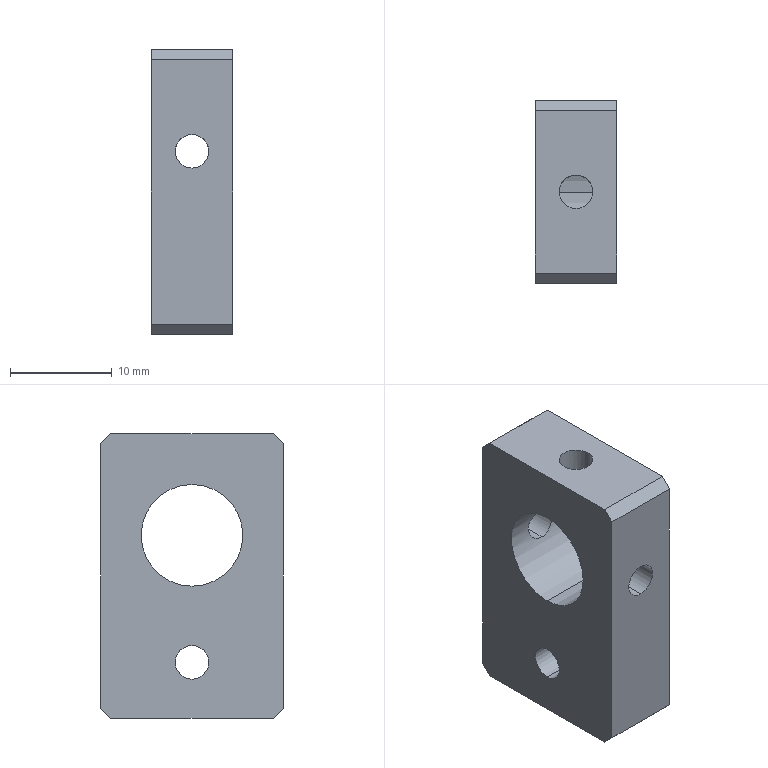Part | SolidWorks | features HoleWzd 3, Chamfer 1, Extrusion 1, ICE 1 | 1 solid | 20 faces | box 8 x 18 x 28 mm | volume 3206 mm3 | cylinder 10 | plane 10 | commonest cylinder face diameters 3.3 x8 10 x2
STEP:
#1=CARTESIAN_POINT('',(0.,-9.,2.35));
#2=VERTEX_POINT('',#1);
#3=CARTESIAN_POINT('',(0.,-9.,5.65));
#4=VERTEX_POINT('',#3);
#5=CARTESIAN_POINT('',(0.,-9.,4.));
#6=DIRECTION('',(0.,1.,0.));
#7=DIRECTION('',(0.,0.,1.));
#8=AXIS2_PLACEMENT_3D('',#5,#6,#7);
#9=CIRCLE('',#8,1.65);
#10=EDGE_CURVE('',#2,#4,#9,.T.);
#11=ORIENTED_EDGE('',*,*,#10,.F.);
#12=CARTESIAN_POINT('',(0.,-4.72,2.35));
#13=VERTEX_POINT('',#12);
#14=CARTESIAN_POINT('',(0.,9.,2.35));
#15=DIRECTION('',(0.,1.,0.));
#16=VECTOR('',#15,1000.);
#17=LINE('',#14,#16);
#18=EDGE_CURVE('',#2,#13,#17,.T.);
#19=ORIENTED_EDGE('',*,*,#18,.T.);
#20=CARTESIAN_POINT('',(0.,-4.72,5.65));
#21=VERTEX_POINT('',#20);
#22=CARTESIAN_POINT('',(0.,-4.72,5.65));
#23=CARTESIAN_POINT('',(-0.1099,-4.72,5.65));
#24=CARTESIAN_POINT('',(-0.2177,-4.724,5.639));
#25=CARTESIAN_POINT('',(-0.4296,-4.738,5.597));
#26=CARTESIAN_POINT('',(-0.5348,-4.749,5.565));
#27=CARTESIAN_POINT('',(-0.7342,-4.776,5.482));
#28=CARTESIAN_POINT('',(-0.8287,-4.791,5.431));
#29=CARTESIAN_POINT('',(-1.007,-4.825,5.311));
#30=CARTESIAN_POINT('',(-1.091,-4.844,5.242));
#31=CARTESIAN_POINT('',(-1.318,-4.898,5.015));
#32=CARTESIAN_POINT('',(-1.441,-4.934,4.833));
#33=CARTESIAN_POINT('',(-1.565,-4.972,4.535));
#34=CARTESIAN_POINT('',(-1.597,-4.983,4.43));
#35=CARTESIAN_POINT('',(-1.639,-4.996,4.217));
#36=CARTESIAN_POINT('',(-1.65,-5.,4.109));
#37=CARTESIAN_POINT('',(-1.65,-5.,3.892));
#38=CARTESIAN_POINT('',(-1.639,-4.996,3.782));
#39=CARTESIAN_POINT('',(-1.597,-4.983,3.57));
#40=CARTESIAN_POINT('',(-1.565,-4.972,3.466));
#41=CARTESIAN_POINT('',(-1.44,-4.934,3.165));
#42=CARTESIAN_POINT('',(-1.318,-4.898,2.984));
#43=CARTESIAN_POINT('',(-1.09,-4.844,2.757));
#44=CARTESIAN_POINT('',(-1.007,-4.825,2.689));
#45=CARTESIAN_POINT('',(-0.8292,-4.791,2.569));
#46=CARTESIAN_POINT('',(-0.7327,-4.775,2.518));
#47=CARTESIAN_POINT('',(-0.5341,-4.749,2.435));
#48=CARTESIAN_POINT('',(-0.4311,-4.738,2.404));
#49=CARTESIAN_POINT('',(-0.2176,-4.724,2.361));
#50=CARTESIAN_POINT('',(-0.1082,-4.72,2.35));
#51=CARTESIAN_POINT('',(0.,-4.72,2.35));
#52=B_SPLINE_CURVE_WITH_KNOTS('',3,(#22,#23,#24,#25,#26,#27,#28,#29,#30,#31,#32,#33,#34,#35,#36,#37,#38,#39,#40,#41,#42,#43,#44,#45,#46,#47,#48,#49,#50,#51),.UNSPECIFIED.,.F.,.F.,(4,2,2,2,2,2,2,2,2,2,2,2,2,2,4),(0.,0.0003247,0.0006494,0.0009741,0.001299,0.001948,0.002273,0.002598,0.002922,0.003247,0.003896,0.004221,0.004546,0.00487,0.005195),.UNSPECIFIED.);
#53=EDGE_CURVE('',#21,#13,#52,.T.);
#54=ORIENTED_EDGE('',*,*,#53,.F.);
#55=CARTESIAN_POINT('',(0.,9.,5.65));
#56=DIRECTION('',(0.,1.,0.));
#57=VECTOR('',#56,1000.);
#58=LINE('',#55,#57);
#59=EDGE_CURVE('',#4,#21,#58,.T.);
#60=ORIENTED_EDGE('',*,*,#59,.F.);
#61=EDGE_LOOP('',(#11,#19,#54,#60));
#62=FACE_OUTER_BOUND('',#61,.T.);
#63=CARTESIAN_POINT('',(0.,9.,4.));
#64=DIRECTION('',(0.,1.,0.));
#65=DIRECTION('',(0.,0.,1.));
#66=AXIS2_PLACEMENT_3D('',#63,#64,#65);
#67=CYLINDRICAL_SURFACE('',#66,1.65);
#68=ADVANCED_FACE('',(#62),#67,.F.);
#69=CARTESIAN_POINT('',(0.,4.72,2.35));
#70=VERTEX_POINT('',#69);
#71=CARTESIAN_POINT('',(0.,4.72,5.65));
#72=VERTEX_POINT('',#71);
#73=CARTESIAN_POINT('',(0.,4.72,2.35));
#74=CARTESIAN_POINT('',(-0.2163,4.72,2.35));
#75=CARTESIAN_POINT('',(-0.4347,4.736,2.394));
#76=CARTESIAN_POINT('',(-0.7332,4.776,2.518));
#77=CARTESIAN_POINT('',(-0.8297,4.791,2.57));
#78=CARTESIAN_POINT('',(-1.008,4.826,2.689));
#79=CARTESIAN_POINT('',(-1.09,4.844,2.757));
#80=CARTESIAN_POINT('',(-1.319,4.899,2.986));
#81=CARTESIAN_POINT('',(-1.44,4.934,3.166));
#82=CARTESIAN_POINT('',(-1.565,4.972,3.467));
#83=CARTESIAN_POINT('',(-1.597,4.983,3.57));
#84=CARTESIAN_POINT('',(-1.639,4.996,3.781));
#85=CARTESIAN_POINT('',(-1.65,5.,3.891));
#86=CARTESIAN_POINT('',(-1.65,5.,4.109));
#87=CARTESIAN_POINT('',(-1.639,4.996,4.217));
#88=CARTESIAN_POINT('',(-1.597,4.983,4.43));
#89=CARTESIAN_POINT('',(-1.565,4.972,4.535));
#90=CARTESIAN_POINT('',(-1.441,4.934,4.833));
#91=CARTESIAN_POINT('',(-1.318,4.898,5.016));
#92=CARTESIAN_POINT('',(-1.091,4.844,5.242));
#93=CARTESIAN_POINT('',(-1.007,4.825,5.312));
#94=CARTESIAN_POINT('',(-0.8285,4.791,5.431));
#95=CARTESIAN_POINT('',(-0.7342,4.776,5.482));
#96=CARTESIAN_POINT('',(-0.5349,4.749,5.565));
#97=CARTESIAN_POINT('',(-0.4296,4.738,5.597));
#98=CARTESIAN_POINT('',(-0.2177,4.724,5.639));
#99=CARTESIAN_POINT('',(-0.1098,4.72,5.65));
#100=CARTESIAN_POINT('',(0.,4.72,5.65));
#101=B_SPLINE_CURVE_WITH_KNOTS('',3,(#73,#74,#75,#76,#77,#78,#79,#80,#81,#82,#83,#84,#85,#86,#87,#88,#89,#90,#91,#92,#93,#94,#95,#96,#97,#98,#99,#100),.UNSPECIFIED.,.F.,.F.,(4,2,2,2,2,2,2,2,2,2,2,2,2,4),(0.005195,0.005844,0.006169,0.006494,0.007143,0.007467,0.007792,0.008117,0.008441,0.009091,0.009415,0.00974,0.01006,0.01039),.UNSPECIFIED.);
#102=EDGE_CURVE('',#70,#72,#101,.T.);
#103=ORIENTED_EDGE('',*,*,#102,.F.);
#104=CARTESIAN_POINT('',(0.,9.,2.35));
#105=VERTEX_POINT('',#104);
#106=CARTESIAN_POINT('',(0.,9.,2.35));
#107=DIRECTION('',(0.,1.,0.));
#108=VECTOR('',#107,1000.);
#109=LINE('',#106,#108);
#110=EDGE_CURVE('',#70,#105,#109,.T.);
#111=ORIENTED_EDGE('',*,*,#110,.T.);
#112=CARTESIAN_POINT('',(0.,9.,5.65));
#113=VERTEX_POINT('',#112);
#114=CARTESIAN_POINT('',(0.,9.,4.));
#115=DIRECTION('',(0.,1.,0.));
#116=DIRECTION('',(0.,0.,1.));
#117=AXIS2_PLACEMENT_3D('',#114,#115,#116);
#118=CIRCLE('',#117,1.65);
#119=EDGE_CURVE('',#105,#113,#118,.T.);
#120=ORIENTED_EDGE('',*,*,#119,.T.);
#121=CARTESIAN_POINT('',(0.,9.,5.65));
#122=DIRECTION('',(0.,1.,0.));
#123=VECTOR('',#122,1000.);
#124=LINE('',#121,#123);
#125=EDGE_CURVE('',#72,#113,#124,.T.);
#126=ORIENTED_EDGE('',*,*,#125,.F.);
#127=EDGE_LOOP('',(#103,#111,#120,#126));
#128=FACE_OUTER_BOUND('',#127,.T.);
#129=CARTESIAN_POINT('',(0.,9.,4.));
#130=DIRECTION('',(0.,1.,0.));
#131=DIRECTION('',(0.,0.,1.));
#132=AXIS2_PLACEMENT_3D('',#129,#130,#131);
#133=CYLINDRICAL_SURFACE('',#132,1.65);
#134=ADVANCED_FACE('',(#128),#133,.F.);
#135=CARTESIAN_POINT('',(-4.,0.,-6.85));
#136=VERTEX_POINT('',#135);
#137=CARTESIAN_POINT('',(-4.,0.,-10.15));
#138=VERTEX_POINT('',#137);
#139=CARTESIAN_POINT('',(-4.,0.,-8.5));
#140=DIRECTION('',(1.,0.,0.));
#141=DIRECTION('',(0.,0.,-1.));
#142=AXIS2_PLACEMENT_3D('',#139,#140,#141);
#143=CIRCLE('',#142,1.65);
#144=EDGE_CURVE('',#136,#138,#143,.T.);
#145=ORIENTED_EDGE('',*,*,#144,.F.);
#146=CARTESIAN_POINT('',(4.,0.,-6.85));
#147=VERTEX_POINT('',#146);
#148=CARTESIAN_POINT('',(4.,0.,-6.85));
#149=DIRECTION('',(1.,0.,0.));
#150=VECTOR('',#149,1000.);
#151=LINE('',#148,#150);
#152=EDGE_CURVE('',#136,#147,#151,.T.);
#153=ORIENTED_EDGE('',*,*,#152,.T.);
#154=CARTESIAN_POINT('',(4.,0.,-10.15));
#155=VERTEX_POINT('',#154);
#156=CARTESIAN_POINT('',(4.,0.,-8.5));
#157=DIRECTION('',(1.,0.,0.));
#158=DIRECTION('',(0.,0.,-1.));
#159=AXIS2_PLACEMENT_3D('',#156,#157,#158);
#160=CIRCLE('',#159,1.65);
#161=EDGE_CURVE('',#147,#155,#160,.T.);
#162=ORIENTED_EDGE('',*,*,#161,.T.);
#163=CARTESIAN_POINT('',(4.,0.,-10.15));
#164=DIRECTION('',(1.,0.,0.));
#165=VECTOR('',#164,1000.);
#166=LINE('',#163,#165);
#167=EDGE_CURVE('',#138,#155,#166,.T.);
#168=ORIENTED_EDGE('',*,*,#167,.F.);
#169=EDGE_LOOP('',(#145,#153,#162,#168));
#170=FACE_OUTER_BOUND('',#169,.T.);
#171=CARTESIAN_POINT('',(4.,0.,-8.5));
#172=DIRECTION('',(1.,0.,0.));
#173=DIRECTION('',(0.,0.,-1.));
#174=AXIS2_PLACEMENT_3D('',#171,#172,#173);
#175=CYLINDRICAL_SURFACE('',#174,1.65);
#176=ADVANCED_FACE('',(#170),#175,.F.);
#177=CARTESIAN_POINT('',(-1.65,0.,9.));
#178=VERTEX_POINT('',#177);
#179=CARTESIAN_POINT('',(1.65,0.,9.));
#180=VERTEX_POINT('',#179);
#181=CARTESIAN_POINT('',(-1.65,0.,9.));
#182=CARTESIAN_POINT('',(-1.65,-0.2164,9.));
#183=CARTESIAN_POINT('',(-1.606,-0.4348,8.985));
#184=CARTESIAN_POINT('',(-1.482,-0.7334,8.947));
#185=CARTESIAN_POINT('',(-1.43,-0.8299,8.931));
#186=CARTESIAN_POINT('',(-1.311,-1.008,8.898));
#187=CARTESIAN_POINT('',(-1.243,-1.091,8.88));
#188=CARTESIAN_POINT('',(-1.014,-1.319,8.825));
#189=CARTESIAN_POINT('',(-0.8342,-1.44,8.789));
#190=CARTESIAN_POINT('',(-0.5334,-1.565,8.749));
#191=CARTESIAN_POINT('',(-0.4303,-1.597,8.738));
#192=CARTESIAN_POINT('',(-0.2186,-1.639,8.724));
#193=CARTESIAN_POINT('',(-0.1086,-1.65,8.72));
#194=CARTESIAN_POINT('',(0.1089,-1.65,8.72));
#195=CARTESIAN_POINT('',(0.2165,-1.639,8.724));
#196=CARTESIAN_POINT('',(0.4297,-1.597,8.738));
#197=CARTESIAN_POINT('',(0.5347,-1.565,8.749));
#198=CARTESIAN_POINT('',(0.8327,-1.441,8.789));
#199=CARTESIAN_POINT('',(1.015,-1.318,8.826));
#200=CARTESIAN_POINT('',(1.242,-1.091,8.88));
#201=CARTESIAN_POINT('',(1.311,-1.007,8.898));
#202=CARTESIAN_POINT('',(1.431,-0.8287,8.932));
#203=CARTESIAN_POINT('',(1.481,-0.7344,8.947));
#204=CARTESIAN_POINT('',(1.565,-0.535,8.972));
#205=CARTESIAN_POINT('',(1.597,-0.4297,8.983));
#206=CARTESIAN_POINT('',(1.639,-0.2177,8.996));
#207=CARTESIAN_POINT('',(1.65,-0.1098,9.));
#208=CARTESIAN_POINT('',(1.65,0.,9.));
#209=B_SPLINE_CURVE_WITH_KNOTS('',3,(#181,#182,#183,#184,#185,#186,#187,#188,#189,#190,#191,#192,#193,#194,#195,#196,#197,#198,#199,#200,#201,#202,#203,#204,#205,#206,#207,#208),.UNSPECIFIED.,.F.,.F.,(4,2,2,2,2,2,2,2,2,2,2,2,2,4),(0.005195,0.005845,0.006169,0.006494,0.007143,0.007468,0.007792,0.008117,0.008442,0.009091,0.009415,0.00974,0.01006,0.01039),.UNSPECIFIED.);
#210=EDGE_CURVE('',#178,#180,#209,.T.);
#211=ORIENTED_EDGE('',*,*,#210,.F.);
#212=CARTESIAN_POINT('',(-1.65,0.,14.));
#213=VERTEX_POINT('',#212);
#214=CARTESIAN_POINT('',(-1.65,0.,14.));
#215=DIRECTION('',(0.,0.,1.));
#216=VECTOR('',#215,1000.);
#217=LINE('',#214,#216);
#218=EDGE_CURVE('',#178,#213,#217,.T.);
#219=ORIENTED_EDGE('',*,*,#218,.T.);
#220=CARTESIAN_POINT('',(1.65,0.,14.));
#221=VERTEX_POINT('',#220);
#222=CARTESIAN_POINT('',(0.,0.,14.));
#223=DIRECTION('',(0.,0.,1.));
#224=DIRECTION('',(1.,0.,0.));
#225=AXIS2_PLACEMENT_3D('',#222,#223,#224);
#226=CIRCLE('',#225,1.65);
#227=EDGE_CURVE('',#213,#221,#226,.T.);
#228=ORIENTED_EDGE('',*,*,#227,.T.);
#229=CARTESIAN_POINT('',(1.65,0.,14.));
#230=DIRECTION('',(0.,0.,1.));
#231=VECTOR('',#230,1000.);
#232=LINE('',#229,#231);
#233=EDGE_CURVE('',#180,#221,#232,.T.);
#234=ORIENTED_EDGE('',*,*,#233,.F.);
#235=EDGE_LOOP('',(#211,#219,#228,#234));
#236=FACE_OUTER_BOUND('',#235,.T.);
#237=CARTESIAN_POINT('',(0.,0.,14.));
#238=DIRECTION('',(0.,0.,1.));
#239=DIRECTION('',(1.,0.,0.));
#240=AXIS2_PLACEMENT_3D('',#237,#238,#239);
#241=CYLINDRICAL_SURFACE('',#240,1.65);
#242=ADVANCED_FACE('',(#236),#241,.F.);
#243=ORIENTED_EDGE('',*,*,#53,.T.);
#244=CARTESIAN_POINT('',(0.,-4.72,2.35));
#245=CARTESIAN_POINT('',(0.2163,-4.72,2.35));
#246=CARTESIAN_POINT('',(0.4347,-4.736,2.394));
#247=CARTESIAN_POINT('',(0.7332,-4.776,2.518));
#248=CARTESIAN_POINT('',(0.8297,-4.791,2.57));
#249=CARTESIAN_POINT('',(1.008,-4.826,2.689));
#250=CARTESIAN_POINT('',(1.09,-4.844,2.757));
#251=CARTESIAN_POINT('',(1.319,-4.899,2.986));
#252=CARTESIAN_POINT('',(1.44,-4.934,3.166));
#253=CARTESIAN_POINT('',(1.565,-4.972,3.467));
#254=CARTESIAN_POINT('',(1.597,-4.983,3.57));
#255=CARTESIAN_POINT('',(1.639,-4.996,3.781));
#256=CARTESIAN_POINT('',(1.65,-5.,3.891));
#257=CARTESIAN_POINT('',(1.65,-5.,4.109));
#258=CARTESIAN_POINT('',(1.639,-4.996,4.217));
#259=CARTESIAN_POINT('',(1.597,-4.983,4.43));
#260=CARTESIAN_POINT('',(1.565,-4.972,4.535));
#261=CARTESIAN_POINT('',(1.441,-4.934,4.833));
#262=CARTESIAN_POINT('',(1.318,-4.898,5.016));
#263=CARTESIAN_POINT('',(1.091,-4.844,5.242));
#264=CARTESIAN_POINT('',(1.007,-4.825,5.312));
#265=CARTESIAN_POINT('',(0.8285,-4.791,5.431));
#266=CARTESIAN_POINT('',(0.7342,-4.776,5.482));
#267=CARTESIAN_POINT('',(0.5349,-4.749,5.565));
#268=CARTESIAN_POINT('',(0.4296,-4.738,5.597));
#269=CARTESIAN_POINT('',(0.2177,-4.724,5.639));
#270=CARTESIAN_POINT('',(0.1098,-4.72,5.65));
#271=CARTESIAN_POINT('',(0.,-4.72,5.65));
#272=B_SPLINE_CURVE_WITH_KNOTS('',3,(#244,#245,#246,#247,#248,#249,#250,#251,#252,#253,#254,#255,#256,#257,#258,#259,#260,#261,#262,#263,#264,#265,#266,#267,#268,#269,#270,#271),.UNSPECIFIED.,.F.,.F.,(4,2,2,2,2,2,2,2,2,2,2,2,2,4),(0.005195,0.005844,0.006169,0.006494,0.007143,0.007467,0.007792,0.008117,0.008441,0.009091,0.009415,0.00974,0.01006,0.01039),.UNSPECIFIED.);
#273=EDGE_CURVE('',#13,#21,#272,.T.);
#274=ORIENTED_EDGE('',*,*,#273,.T.);
#275=EDGE_LOOP('',(#243,#274));
#276=FACE_BOUND('',#275,.T.);
#277=CARTESIAN_POINT('',(-4.,0.,9.));
#278=VERTEX_POINT('',#277);
#279=CARTESIAN_POINT('',(-4.,0.,-1.));
#280=VERTEX_POINT('',#279);
#281=CARTESIAN_POINT('',(-4.,0.,4.));
#282=DIRECTION('',(1.,0.,0.));
#283=DIRECTION('',(0.,0.,-1.));
#284=AXIS2_PLACEMENT_3D('',#281,#282,#283);
#285=CIRCLE('',#284,5.);
#286=EDGE_CURVE('',#278,#280,#285,.T.);
#287=ORIENTED_EDGE('',*,*,#286,.F.);
#288=CARTESIAN_POINT('',(-4.,0.,9.));
#289=DIRECTION('',(1.,0.,0.));
#290=VECTOR('',#289,1000.);
#291=LINE('',#288,#290);
#292=EDGE_CURVE('',#278,#178,#291,.T.);
#293=ORIENTED_EDGE('',*,*,#292,.T.);
#294=ORIENTED_EDGE('',*,*,#210,.T.);
#295=CARTESIAN_POINT('',(4.,0.,9.));
#296=VERTEX_POINT('',#295);
#297=CARTESIAN_POINT('',(-4.,0.,9.));
#298=DIRECTION('',(1.,0.,0.));
#299=VECTOR('',#298,1000.);
#300=LINE('',#297,#299);
#301=EDGE_CURVE('',#180,#296,#300,.T.);
#302=ORIENTED_EDGE('',*,*,#301,.T.);
#303=CARTESIAN_POINT('',(4.,0.,-1.));
#304=VERTEX_POINT('',#303);
#305=CARTESIAN_POINT('',(4.,0.,4.));
#306=DIRECTION('',(1.,0.,0.));
#307=DIRECTION('',(0.,0.,-1.));
#308=AXIS2_PLACEMENT_3D('',#305,#306,#307);
#309=CIRCLE('',#308,5.);
#310=EDGE_CURVE('',#296,#304,#309,.T.);
#311=ORIENTED_EDGE('',*,*,#310,.T.);
#312=CARTESIAN_POINT('',(-4.,0.,-1.));
#313=DIRECTION('',(1.,0.,0.));
#314=VECTOR('',#313,1000.);
#315=LINE('',#312,#314);
#316=EDGE_CURVE('',#280,#304,#315,.T.);
#317=ORIENTED_EDGE('',*,*,#316,.F.);
#318=EDGE_LOOP('',(#287,#293,#294,#302,#311,#317));
#319=FACE_OUTER_BOUND('',#318,.T.);
#320=CARTESIAN_POINT('',(-4.,0.,4.));
#321=DIRECTION('',(1.,0.,0.));
#322=DIRECTION('',(0.,0.,-1.));
#323=AXIS2_PLACEMENT_3D('',#320,#321,#322);
#324=CYLINDRICAL_SURFACE('',#323,5.);
#325=ADVANCED_FACE('',(#276,#319),#324,.F.);
#326=CARTESIAN_POINT('',(0.,0.,14.));
#327=DIRECTION('',(0.,0.,1.));
#328=DIRECTION('',(1.,0.,0.));
#329=AXIS2_PLACEMENT_3D('',#326,#327,#328);
#330=CIRCLE('',#329,1.65);
#331=EDGE_CURVE('',#221,#213,#330,.T.);
#332=ORIENTED_EDGE('',*,*,#331,.F.);
#333=ORIENTED_EDGE('',*,*,#227,.F.);
#334=EDGE_LOOP('',(#332,#333));
#335=FACE_BOUND('',#334,.T.);
#336=CARTESIAN_POINT('',(-4.,8.,14.));
#337=VERTEX_POINT('',#336);
#338=CARTESIAN_POINT('',(-4.,-8.,14.));
#339=VERTEX_POINT('',#338);
#340=CARTESIAN_POINT('',(-4.,-9.,14.));
#341=DIRECTION('',(0.,-1.,0.));
#342=VECTOR('',#341,1000.);
#343=LINE('',#340,#342);
#344=EDGE_CURVE('',#337,#339,#343,.T.);
#345=ORIENTED_EDGE('',*,*,#344,.T.);
#346=CARTESIAN_POINT('',(4.,-8.,14.));
#347=VERTEX_POINT('',#346);
#348=CARTESIAN_POINT('',(4.,-8.,14.));
#349=DIRECTION('',(1.,0.,0.));
#350=VECTOR('',#349,1000.);
#351=LINE('',#348,#350);
#352=EDGE_CURVE('',#339,#347,#351,.T.);
#353=ORIENTED_EDGE('',*,*,#352,.T.);
#354=CARTESIAN_POINT('',(4.,8.,14.));
#355=VERTEX_POINT('',#354);
#356=CARTESIAN_POINT('',(4.,-9.,14.));
#357=DIRECTION('',(0.,-1.,0.));
#358=VECTOR('',#357,1000.);
#359=LINE('',#356,#358);
#360=EDGE_CURVE('',#355,#347,#359,.T.);
#361=ORIENTED_EDGE('',*,*,#360,.F.);
#362=CARTESIAN_POINT('',(4.,8.,14.));
#363=DIRECTION('',(-1.,0.,0.));
#364=VECTOR('',#363,1000.);
#365=LINE('',#362,#364);
#366=EDGE_CURVE('',#355,#337,#365,.T.);
#367=ORIENTED_EDGE('',*,*,#366,.T.);
#368=EDGE_LOOP('',(#345,#353,#361,#367));
#369=FACE_OUTER_BOUND('',#368,.T.);
#370=CARTESIAN_POINT('',(4.,-9.,14.));
#371=DIRECTION('',(0.,0.,-1.));
#372=DIRECTION('',(-1.,0.,0.));
#373=AXIS2_PLACEMENT_3D('',#370,#371,#372);
#374=PLANE('',#373);
#375=ADVANCED_FACE('',(#335,#369),#374,.F.);
#376=CARTESIAN_POINT('',(0.,-9.,4.));
#377=DIRECTION('',(0.,1.,0.));
#378=DIRECTION('',(0.,0.,1.));
#379=AXIS2_PLACEMENT_3D('',#376,#377,#378);
#380=CIRCLE('',#379,1.65);
#381=EDGE_CURVE('',#4,#2,#380,.T.);
#382=ORIENTED_EDGE('',*,*,#381,.T.);
#383=ORIENTED_EDGE('',*,*,#10,.T.);
#384=EDGE_LOOP('',(#382,#383));
#385=FACE_BOUND('',#384,.T.);
#386=CARTESIAN_POINT('',(-4.,-9.,13.));
#387=VERTEX_POINT('',#386);
#388=CARTESIAN_POINT('',(-4.,-9.,-13.));
#389=VERTEX_POINT('',#388);
#390=CARTESIAN_POINT('',(-4.,-9.,-14.));
#391=DIRECTION('',(0.,0.,-1.));
#392=VECTOR('',#391,1000.);
#393=LINE('',#390,#392);
#394=EDGE_CURVE('',#387,#389,#393,.T.);
#395=ORIENTED_EDGE('',*,*,#394,.T.);
#396=CARTESIAN_POINT('',(4.,-9.,-13.));
#397=VERTEX_POINT('',#396);
#398=CARTESIAN_POINT('',(4.,-9.,-13.));
#399=DIRECTION('',(1.,0.,0.));
#400=VECTOR('',#399,1000.);
#401=LINE('',#398,#400);
#402=EDGE_CURVE('',#389,#397,#401,.T.);
#403=ORIENTED_EDGE('',*,*,#402,.T.);
#404=CARTESIAN_POINT('',(4.,-9.,13.));
#405=VERTEX_POINT('',#404);
#406=CARTESIAN_POINT('',(4.,-9.,-14.));
#407=DIRECTION('',(0.,0.,-1.));
#408=VECTOR('',#407,1000.);
#409=LINE('',#406,#408);
#410=EDGE_CURVE('',#405,#397,#409,.T.);
#411=ORIENTED_EDGE('',*,*,#410,.F.);
#412=CARTESIAN_POINT('',(4.,-9.,13.));
#413=DIRECTION('',(-1.,0.,0.));
#414=VECTOR('',#413,1000.);
#415=LINE('',#412,#414);
#416=EDGE_CURVE('',#405,#387,#415,.T.);
#417=ORIENTED_EDGE('',*,*,#416,.T.);
#418=EDGE_LOOP('',(#395,#403,#411,#417));
#419=FACE_OUTER_BOUND('',#418,.T.);
#420=CARTESIAN_POINT('',(4.,-9.,-14.));
#421=DIRECTION('',(0.,1.,0.));
#422=DIRECTION('',(0.,0.,1.));
#423=AXIS2_PLACEMENT_3D('',#420,#421,#422);
#424=PLANE('',#423);
#425=ADVANCED_FACE('',(#385,#419),#424,.F.);
#426=CARTESIAN_POINT('',(4.,-8.,-14.));
#427=VERTEX_POINT('',#426);
#428=CARTESIAN_POINT('',(4.,8.,-14.));
#429=VERTEX_POINT('',#428);
#430=CARTESIAN_POINT('',(4.,-9.,-14.));
#431=DIRECTION('',(0.,1.,0.));
#432=VECTOR('',#431,1000.);
#433=LINE('',#430,#432);
#434=EDGE_CURVE('',#427,#429,#433,.T.);
#435=ORIENTED_EDGE('',*,*,#434,.F.);
#436=CARTESIAN_POINT('',(-4.,-8.,-14.));
#437=VERTEX_POINT('',#436);
#438=CARTESIAN_POINT('',(4.,-8.,-14.));
#439=DIRECTION('',(-1.,0.,0.));
#440=VECTOR('',#439,1000.);
#441=LINE('',#438,#440);
#442=EDGE_CURVE('',#427,#437,#441,.T.);
#443=ORIENTED_EDGE('',*,*,#442,.T.);
#444=CARTESIAN_POINT('',(-4.,8.,-14.));
#445=VERTEX_POINT('',#444);
#446=CARTESIAN_POINT('',(-4.,-9.,-14.));
#447=DIRECTION('',(0.,1.,0.));
#448=VECTOR('',#447,1000.);
#449=LINE('',#446,#448);
#450=EDGE_CURVE('',#437,#445,#449,.T.);
#451=ORIENTED_EDGE('',*,*,#450,.T.);
#452=CARTESIAN_POINT('',(4.,8.,-14.));
#453=DIRECTION('',(1.,0.,0.));
#454=VECTOR('',#453,1000.);
#455=LINE('',#452,#454);
#456=EDGE_CURVE('',#445,#429,#455,.T.);
#457=ORIENTED_EDGE('',*,*,#456,.T.);
#458=EDGE_LOOP('',(#435,#443,#451,#457));
#459=FACE_OUTER_BOUND('',#458,.T.);
#460=CARTESIAN_POINT('',(4.,-9.,-14.));
#461=DIRECTION('',(0.,0.,1.));
#462=DIRECTION('',(1.,0.,0.));
#463=AXIS2_PLACEMENT_3D('',#460,#461,#462);
#464=PLANE('',#463);
#465=ADVANCED_FACE('',(#459),#464,.F.);
#466=CARTESIAN_POINT('',(0.,9.,4.));
#467=DIRECTION('',(0.,1.,0.));
#468=DIRECTION('',(0.,0.,1.));
#469=AXIS2_PLACEMENT_3D('',#466,#467,#468);
#470=CIRCLE('',#469,1.65);
#471=EDGE_CURVE('',#113,#105,#470,.T.);
#472=ORIENTED_EDGE('',*,*,#471,.F.);
#473=ORIENTED_EDGE('',*,*,#119,.F.);
#474=EDGE_LOOP('',(#472,#473));
#475=FACE_BOUND('',#474,.T.);
#476=CARTESIAN_POINT('',(4.,9.,-13.));
#477=VERTEX_POINT('',#476);
#478=CARTESIAN_POINT('',(4.,9.,13.));
#479=VERTEX_POINT('',#478);
#480=CARTESIAN_POINT('',(4.,9.,-14.));
#481=DIRECTION('',(0.,0.,1.));
#482=VECTOR('',#481,1000.);
#483=LINE('',#480,#482);
#484=EDGE_CURVE('',#477,#479,#483,.T.);
#485=ORIENTED_EDGE('',*,*,#484,.F.);
#486=CARTESIAN_POINT('',(-4.,9.,-13.));
#487=VERTEX_POINT('',#486);
#488=CARTESIAN_POINT('',(4.,9.,-13.));
#489=DIRECTION('',(-1.,0.,0.));
#490=VECTOR('',#489,1000.);
#491=LINE('',#488,#490);
#492=EDGE_CURVE('',#477,#487,#491,.T.);
#493=ORIENTED_EDGE('',*,*,#492,.T.);
#494=CARTESIAN_POINT('',(-4.,9.,13.));
#495=VERTEX_POINT('',#494);
#496=CARTESIAN_POINT('',(-4.,9.,-14.));
#497=DIRECTION('',(0.,0.,1.));
#498=VECTOR('',#497,1000.);
#499=LINE('',#496,#498);
#500=EDGE_CURVE('',#487,#495,#499,.T.);
#501=ORIENTED_EDGE('',*,*,#500,.T.);
#502=CARTESIAN_POINT('',(4.,9.,13.));
#503=DIRECTION('',(1.,0.,0.));
#504=VECTOR('',#503,1000.);
#505=LINE('',#502,#504);
#506=EDGE_CURVE('',#495,#479,#505,.T.);
#507=ORIENTED_EDGE('',*,*,#506,.T.);
#508=EDGE_LOOP('',(#485,#493,#501,#507));
#509=FACE_OUTER_BOUND('',#508,.T.);
#510=CARTESIAN_POINT('',(4.,9.,-14.));
#511=DIRECTION('',(0.,-1.,0.));
#512=DIRECTION('',(0.,0.,-1.));
#513=AXIS2_PLACEMENT_3D('',#510,#511,#512);
#514=PLANE('',#513);
#515=ADVANCED_FACE('',(#475,#509),#514,.F.);
#516=CARTESIAN_POINT('',(4.,0.,-8.5));
#517=DIRECTION('',(1.,0.,0.));
#518=DIRECTION('',(0.,0.,-1.));
#519=AXIS2_PLACEMENT_3D('',#516,#517,#518);
#520=CIRCLE('',#519,1.65);
#521=EDGE_CURVE('',#155,#147,#520,.T.);
#522=ORIENTED_EDGE('',*,*,#521,.F.);
#523=ORIENTED_EDGE('',*,*,#161,.F.);
#524=EDGE_LOOP('',(#522,#523));
#525=FACE_BOUND('',#524,.T.);
#526=CARTESIAN_POINT('',(4.,0.,4.));
#527=DIRECTION('',(1.,0.,0.));
#528=DIRECTION('',(0.,0.,-1.));
#529=AXIS2_PLACEMENT_3D('',#526,#527,#528);
#530=CIRCLE('',#529,5.);
#531=EDGE_CURVE('',#304,#296,#530,.T.);
#532=ORIENTED_EDGE('',*,*,#531,.F.);
#533=ORIENTED_EDGE('',*,*,#310,.F.);
#534=EDGE_LOOP('',(#532,#533));
#535=FACE_BOUND('',#534,.T.);
#536=ORIENTED_EDGE('',*,*,#410,.T.);
#537=CARTESIAN_POINT('',(4.,-11.,-11.));
#538=DIRECTION('',(0.,0.7071,-0.7071));
#539=VECTOR('',#538,1000.);
#540=LINE('',#537,#539);
#541=EDGE_CURVE('',#397,#427,#540,.T.);
#542=ORIENTED_EDGE('',*,*,#541,.T.);
#543=ORIENTED_EDGE('',*,*,#434,.T.);
#544=CARTESIAN_POINT('',(4.,11.,-11.));
#545=DIRECTION('',(0.,0.7071,0.7071));
#546=VECTOR('',#545,1000.);
#547=LINE('',#544,#546);
#548=EDGE_CURVE('',#429,#477,#547,.T.);
#549=ORIENTED_EDGE('',*,*,#548,.T.);
#550=ORIENTED_EDGE('',*,*,#484,.T.);
#551=CARTESIAN_POINT('',(4.,11.,11.));
#552=DIRECTION('',(0.,-0.7071,0.7071));
#553=VECTOR('',#552,1000.);
#554=LINE('',#551,#553);
#555=EDGE_CURVE('',#479,#355,#554,.T.);
#556=ORIENTED_EDGE('',*,*,#555,.T.);
#557=ORIENTED_EDGE('',*,*,#360,.T.);
#558=CARTESIAN_POINT('',(4.,-11.,11.));
#559=DIRECTION('',(0.,-0.7071,-0.7071));
#560=VECTOR('',#559,1000.);
#561=LINE('',#558,#560);
#562=EDGE_CURVE('',#347,#405,#561,.T.);
#563=ORIENTED_EDGE('',*,*,#562,.T.);
#564=EDGE_LOOP('',(#536,#542,#543,#549,#550,#556,#557,#563));
#565=FACE_OUTER_BOUND('',#564,.T.);
#566=CARTESIAN_POINT('',(4.,0.,0.));
#567=DIRECTION('',(1.,0.,0.));
#568=DIRECTION('',(0.,0.,-1.));
#569=AXIS2_PLACEMENT_3D('',#566,#567,#568);
#570=PLANE('',#569);
#571=ADVANCED_FACE('',(#525,#535,#565),#570,.T.);
#572=CARTESIAN_POINT('',(-4.,0.,-8.5));
#573=DIRECTION('',(1.,0.,0.));
#574=DIRECTION('',(0.,0.,-1.));
#575=AXIS2_PLACEMENT_3D('',#572,#573,#574);
#576=CIRCLE('',#575,1.65);
#577=EDGE_CURVE('',#138,#136,#576,.T.);
#578=ORIENTED_EDGE('',*,*,#577,.T.);
#579=ORIENTED_EDGE('',*,*,#144,.T.);
#580=EDGE_LOOP('',(#578,#579));
#581=FACE_BOUND('',#580,.T.);
#582=CARTESIAN_POINT('',(-4.,0.,4.));
#583=DIRECTION('',(1.,0.,0.));
#584=DIRECTION('',(0.,0.,-1.));
#585=AXIS2_PLACEMENT_3D('',#582,#583,#584);
#586=CIRCLE('',#585,5.);
#587=EDGE_CURVE('',#280,#278,#586,.T.);
#588=ORIENTED_EDGE('',*,*,#587,.T.);
#589=ORIENTED_EDGE('',*,*,#286,.T.);
#590=EDGE_LOOP('',(#588,#589));
#591=FACE_BOUND('',#590,.T.);
#592=ORIENTED_EDGE('',*,*,#450,.F.);
#593=CARTESIAN_POINT('',(-4.,-8.,-14.));
#594=DIRECTION('',(0.,-0.7071,0.7071));
#595=VECTOR('',#594,1000.);
#596=LINE('',#593,#595);
#597=EDGE_CURVE('',#437,#389,#596,.T.);
#598=ORIENTED_EDGE('',*,*,#597,.T.);
#599=ORIENTED_EDGE('',*,*,#394,.F.);
#600=CARTESIAN_POINT('',(-4.,-9.,13.));
#601=DIRECTION('',(0.,0.7071,0.7071));
#602=VECTOR('',#601,1000.);
#603=LINE('',#600,#602);
#604=EDGE_CURVE('',#387,#339,#603,.T.);
#605=ORIENTED_EDGE('',*,*,#604,.T.);
#606=ORIENTED_EDGE('',*,*,#344,.F.);
#607=CARTESIAN_POINT('',(-4.,8.,14.));
#608=DIRECTION('',(0.,0.7071,-0.7071));
#609=VECTOR('',#608,1000.);
#610=LINE('',#607,#609);
#611=EDGE_CURVE('',#337,#495,#610,.T.);
#612=ORIENTED_EDGE('',*,*,#611,.T.);
#613=ORIENTED_EDGE('',*,*,#500,.F.);
#614=CARTESIAN_POINT('',(-4.,9.,-13.));
#615=DIRECTION('',(0.,-0.7071,-0.7071));
#616=VECTOR('',#615,1000.);
#617=LINE('',#614,#616);
#618=EDGE_CURVE('',#487,#445,#617,.T.);
#619=ORIENTED_EDGE('',*,*,#618,.T.);
#620=EDGE_LOOP('',(#592,#598,#599,#605,#606,#612,#613,#619));
#621=FACE_OUTER_BOUND('',#620,.T.);
#622=CARTESIAN_POINT('',(-4.,0.,0.));
#623=DIRECTION('',(1.,0.,0.));
#624=DIRECTION('',(0.,0.,-1.));
#625=AXIS2_PLACEMENT_3D('',#622,#623,#624);
#626=PLANE('',#625);
#627=ADVANCED_FACE('',(#581,#591,#621),#626,.F.);
#628=ORIENTED_EDGE('',*,*,#292,.F.);
#629=ORIENTED_EDGE('',*,*,#587,.F.);
#630=ORIENTED_EDGE('',*,*,#316,.T.);
#631=ORIENTED_EDGE('',*,*,#531,.T.);
#632=ORIENTED_EDGE('',*,*,#301,.F.);
#633=CARTESIAN_POINT('',(1.65,0.,9.));
#634=CARTESIAN_POINT('',(1.65,0.1098,9.));
#635=CARTESIAN_POINT('',(1.639,0.2177,8.996));
#636=CARTESIAN_POINT('',(1.597,0.4297,8.983));
#637=CARTESIAN_POINT('',(1.565,0.5349,8.972));
#638=CARTESIAN_POINT('',(1.481,0.7344,8.947));
#639=CARTESIAN_POINT('',(1.431,0.8289,8.932));
#640=CARTESIAN_POINT('',(1.311,1.008,8.898));
#641=CARTESIAN_POINT('',(1.242,1.092,8.88));
#642=CARTESIAN_POINT('',(1.015,1.318,8.826));
#643=CARTESIAN_POINT('',(0.8323,1.441,8.789));
#644=CARTESIAN_POINT('',(0.535,1.565,8.749));
#645=CARTESIAN_POINT('',(0.4302,1.597,8.738));
#646=CARTESIAN_POINT('',(0.2169,1.639,8.724));
#647=CARTESIAN_POINT('',(0.1093,1.65,8.72));
#648=CARTESIAN_POINT('',(-0.1077,1.65,8.72));
#649=CARTESIAN_POINT('',(-0.2179,1.639,8.724));
#650=CARTESIAN_POINT('',(-0.4302,1.597,8.738));
#651=CARTESIAN_POINT('',(-0.5334,1.565,8.749));
#652=CARTESIAN_POINT('',(-0.8346,1.44,8.789));
#653=CARTESIAN_POINT('',(-1.015,1.318,8.826));
#654=CARTESIAN_POINT('',(-1.243,1.09,8.88));
#655=CARTESIAN_POINT('',(-1.311,1.008,8.898));
#656=CARTESIAN_POINT('',(-1.43,0.8295,8.932));
#657=CARTESIAN_POINT('',(-1.482,0.7329,8.947));
#658=CARTESIAN_POINT('',(-1.565,0.5342,8.972));
#659=CARTESIAN_POINT('',(-1.596,0.4312,8.983));
#660=CARTESIAN_POINT('',(-1.639,0.2176,8.996));
#661=CARTESIAN_POINT('',(-1.65,0.1082,9.));
#662=CARTESIAN_POINT('',(-1.65,0.,9.));
#663=B_SPLINE_CURVE_WITH_KNOTS('',3,(#633,#634,#635,#636,#637,#638,#639,#640,#641,#642,#643,#644,#645,#646,#647,#648,#649,#650,#651,#652,#653,#654,#655,#656,#657,#658,#659,#660,#661,#662),.UNSPECIFIED.,.F.,.F.,(4,2,2,2,2,2,2,2,2,2,2,2,2,2,4),(0.,0.0003247,0.0006494,0.0009741,0.001299,0.001948,0.002273,0.002598,0.002922,0.003247,0.003896,0.004221,0.004546,0.004871,0.005195),.UNSPECIFIED.);
#664=EDGE_CURVE('',#180,#178,#663,.T.);
#665=ORIENTED_EDGE('',*,*,#664,.T.);
#666=EDGE_LOOP('',(#628,#629,#630,#631,#632,#665));
#667=FACE_OUTER_BOUND('',#666,.T.);
#668=CARTESIAN_POINT('',(0.,4.72,5.65));
#669=CARTESIAN_POINT('',(0.1099,4.72,5.65));
#670=CARTESIAN_POINT('',(0.2177,4.724,5.639));
#671=CARTESIAN_POINT('',(0.4296,4.738,5.597));
#672=CARTESIAN_POINT('',(0.5348,4.749,5.565));
#673=CARTESIAN_POINT('',(0.7342,4.776,5.482));
#674=CARTESIAN_POINT('',(0.8287,4.791,5.431));
#675=CARTESIAN_POINT('',(1.007,4.825,5.311));
#676=CARTESIAN_POINT('',(1.091,4.844,5.242));
#677=CARTESIAN_POINT('',(1.318,4.898,5.015));
#678=CARTESIAN_POINT('',(1.441,4.934,4.833));
#679=CARTESIAN_POINT('',(1.565,4.972,4.535));
#680=CARTESIAN_POINT('',(1.597,4.983,4.43));
#681=CARTESIAN_POINT('',(1.639,4.996,4.217));
#682=CARTESIAN_POINT('',(1.65,5.,4.109));
#683=CARTESIAN_POINT('',(1.65,5.,3.892));
#684=CARTESIAN_POINT('',(1.639,4.996,3.782));
#685=CARTESIAN_POINT('',(1.597,4.983,3.57));
#686=CARTESIAN_POINT('',(1.565,4.972,3.466));
#687=CARTESIAN_POINT('',(1.44,4.934,3.165));
#688=CARTESIAN_POINT('',(1.318,4.898,2.984));
#689=CARTESIAN_POINT('',(1.09,4.844,2.757));
#690=CARTESIAN_POINT('',(1.007,4.825,2.689));
#691=CARTESIAN_POINT('',(0.8292,4.791,2.569));
#692=CARTESIAN_POINT('',(0.7327,4.775,2.518));
#693=CARTESIAN_POINT('',(0.5341,4.749,2.435));
#694=CARTESIAN_POINT('',(0.4311,4.738,2.404));
#695=CARTESIAN_POINT('',(0.2176,4.724,2.361));
#696=CARTESIAN_POINT('',(0.1082,4.72,2.35));
#697=CARTESIAN_POINT('',(0.,4.72,2.35));
#698=B_SPLINE_CURVE_WITH_KNOTS('',3,(#668,#669,#670,#671,#672,#673,#674,#675,#676,#677,#678,#679,#680,#681,#682,#683,#684,#685,#686,#687,#688,#689,#690,#691,#692,#693,#694,#695,#696,#697),.UNSPECIFIED.,.F.,.F.,(4,2,2,2,2,2,2,2,2,2,2,2,2,2,4),(0.,0.0003247,0.0006494,0.0009741,0.001299,0.001948,0.002273,0.002598,0.002922,0.003247,0.003896,0.004221,0.004546,0.00487,0.005195),.UNSPECIFIED.);
#699=EDGE_CURVE('',#72,#70,#698,.T.);
#700=ORIENTED_EDGE('',*,*,#699,.T.);
#701=ORIENTED_EDGE('',*,*,#102,.T.);
#702=EDGE_LOOP('',(#700,#701));
#703=FACE_BOUND('',#702,.T.);
#704=CARTESIAN_POINT('',(-4.,0.,4.));
#705=DIRECTION('',(1.,0.,0.));
#706=DIRECTION('',(0.,0.,-1.));
#707=AXIS2_PLACEMENT_3D('',#704,#705,#706);
#708=CYLINDRICAL_SURFACE('',#707,5.);
#709=ADVANCED_FACE('',(#667,#703),#708,.F.);
#710=ORIENTED_EDGE('',*,*,#218,.F.);
#711=ORIENTED_EDGE('',*,*,#664,.F.);
#712=ORIENTED_EDGE('',*,*,#233,.T.);
#713=ORIENTED_EDGE('',*,*,#331,.T.);
#714=EDGE_LOOP('',(#710,#711,#712,#713));
#715=FACE_OUTER_BOUND('',#714,.T.);
#716=CARTESIAN_POINT('',(0.,0.,14.));
#717=DIRECTION('',(0.,0.,1.));
#718=DIRECTION('',(1.,0.,0.));
#719=AXIS2_PLACEMENT_3D('',#716,#717,#718);
#720=CYLINDRICAL_SURFACE('',#719,1.65);
#721=ADVANCED_FACE('',(#715),#720,.F.);
#722=ORIENTED_EDGE('',*,*,#152,.F.);
#723=ORIENTED_EDGE('',*,*,#577,.F.);
#724=ORIENTED_EDGE('',*,*,#167,.T.);
#725=ORIENTED_EDGE('',*,*,#521,.T.);
#726=EDGE_LOOP('',(#722,#723,#724,#725));
#727=FACE_OUTER_BOUND('',#726,.T.);
#728=CARTESIAN_POINT('',(4.,0.,-8.5));
#729=DIRECTION('',(1.,0.,0.));
#730=DIRECTION('',(0.,0.,-1.));
#731=AXIS2_PLACEMENT_3D('',#728,#729,#730);
#732=CYLINDRICAL_SURFACE('',#731,1.65);
#733=ADVANCED_FACE('',(#727),#732,.F.);
#734=ORIENTED_EDGE('',*,*,#110,.F.);
#735=ORIENTED_EDGE('',*,*,#699,.F.);
#736=ORIENTED_EDGE('',*,*,#125,.T.);
#737=ORIENTED_EDGE('',*,*,#471,.T.);
#738=EDGE_LOOP('',(#734,#735,#736,#737));
#739=FACE_OUTER_BOUND('',#738,.T.);
#740=CARTESIAN_POINT('',(0.,9.,4.));
#741=DIRECTION('',(0.,1.,0.));
#742=DIRECTION('',(0.,0.,1.));
#743=AXIS2_PLACEMENT_3D('',#740,#741,#742);
#744=CYLINDRICAL_SURFACE('',#743,1.65);
#745=ADVANCED_FACE('',(#739),#744,.F.);
#746=ORIENTED_EDGE('',*,*,#18,.F.);
#747=ORIENTED_EDGE('',*,*,#381,.F.);
#748=ORIENTED_EDGE('',*,*,#59,.T.);
#749=ORIENTED_EDGE('',*,*,#273,.F.);
#750=EDGE_LOOP('',(#746,#747,#748,#749));
#751=FACE_OUTER_BOUND('',#750,.T.);
#752=CARTESIAN_POINT('',(0.,9.,4.));
#753=DIRECTION('',(0.,1.,0.));
#754=DIRECTION('',(0.,0.,1.));
#755=AXIS2_PLACEMENT_3D('',#752,#753,#754);
#756=CYLINDRICAL_SURFACE('',#755,1.65);
#757=ADVANCED_FACE('',(#751),#756,.F.);
#758=ORIENTED_EDGE('',*,*,#541,.F.);
#759=ORIENTED_EDGE('',*,*,#402,.F.);
#760=ORIENTED_EDGE('',*,*,#597,.F.);
#761=ORIENTED_EDGE('',*,*,#442,.F.);
#762=EDGE_LOOP('',(#758,#759,#760,#761));
#763=FACE_OUTER_BOUND('',#762,.T.);
#764=CARTESIAN_POINT('',(4.,-8.,-14.));
#765=DIRECTION('',(0.,0.7071,0.7071));
#766=DIRECTION('',(-1.,0.,0.));
#767=AXIS2_PLACEMENT_3D('',#764,#765,#766);
#768=PLANE('',#767);
#769=ADVANCED_FACE('',(#763),#768,.F.);
#770=ORIENTED_EDGE('',*,*,#548,.F.);
#771=ORIENTED_EDGE('',*,*,#456,.F.);
#772=ORIENTED_EDGE('',*,*,#618,.F.);
#773=ORIENTED_EDGE('',*,*,#492,.F.);
#774=EDGE_LOOP('',(#770,#771,#772,#773));
#775=FACE_OUTER_BOUND('',#774,.T.);
#776=CARTESIAN_POINT('',(4.,9.,-13.));
#777=DIRECTION('',(0.,-0.7071,0.7071));
#778=DIRECTION('',(-1.,0.,0.));
#779=AXIS2_PLACEMENT_3D('',#776,#777,#778);
#780=PLANE('',#779);
#781=ADVANCED_FACE('',(#775),#780,.F.);
#782=ORIENTED_EDGE('',*,*,#562,.F.);
#783=ORIENTED_EDGE('',*,*,#352,.F.);
#784=ORIENTED_EDGE('',*,*,#604,.F.);
#785=ORIENTED_EDGE('',*,*,#416,.F.);
#786=EDGE_LOOP('',(#782,#783,#784,#785));
#787=FACE_OUTER_BOUND('',#786,.T.);
#788=CARTESIAN_POINT('',(4.,-9.,13.));
#789=DIRECTION('',(0.,0.7071,-0.7071));
#790=DIRECTION('',(-1.,0.,0.));
#791=AXIS2_PLACEMENT_3D('',#788,#789,#790);
#792=PLANE('',#791);
#793=ADVANCED_FACE('',(#787),#792,.F.);
#794=ORIENTED_EDGE('',*,*,#555,.F.);
#795=ORIENTED_EDGE('',*,*,#506,.F.);
#796=ORIENTED_EDGE('',*,*,#611,.F.);
#797=ORIENTED_EDGE('',*,*,#366,.F.);
#798=EDGE_LOOP('',(#794,#795,#796,#797));
#799=FACE_OUTER_BOUND('',#798,.T.);
#800=CARTESIAN_POINT('',(4.,8.,14.));
#801=DIRECTION('',(0.,-0.7071,-0.7071));
#802=DIRECTION('',(-1.,0.,0.));
#803=AXIS2_PLACEMENT_3D('',#800,#801,#802);
#804=PLANE('',#803);
#805=ADVANCED_FACE('',(#799),#804,.F.);
#806=CLOSED_SHELL('',(#68,#134,#176,#242,#325,#375,#425,#465,#515,#571,#627,#709,#721,#733,#745,#757,#769,#781,#793,#805));
#807=MANIFOLD_SOLID_BREP('',#806);
#808=CARTESIAN_POINT('',(0.,0.,0.));
#809=DIRECTION('',(0.,0.,1.));
#810=DIRECTION('',(1.,0.,0.));
#811=AXIS2_PLACEMENT_3D('',#808,#809,#810);
#812=(LENGTH_UNIT()NAMED_UNIT(*)SI_UNIT(.MILLI.,.METRE.));
#813=UNCERTAINTY_MEASURE_WITH_UNIT(LENGTH_MEASURE(0.00001),#812,'','');
#814=(NAMED_UNIT(*)PLANE_ANGLE_UNIT()SI_UNIT($,.RADIAN.));
#815=(NAMED_UNIT(*)SI_UNIT($,.STERADIAN.)SOLID_ANGLE_UNIT());
#816=(GEOMETRIC_REPRESENTATION_CONTEXT(3)GLOBAL_UNCERTAINTY_ASSIGNED_CONTEXT((#813))GLOBAL_UNIT_ASSIGNED_CONTEXT((#812,#814,#815))REPRESENTATION_CONTEXT('',''));
#817=ADVANCED_BREP_SHAPE_REPRESENTATION('',(#807,#811),#816);